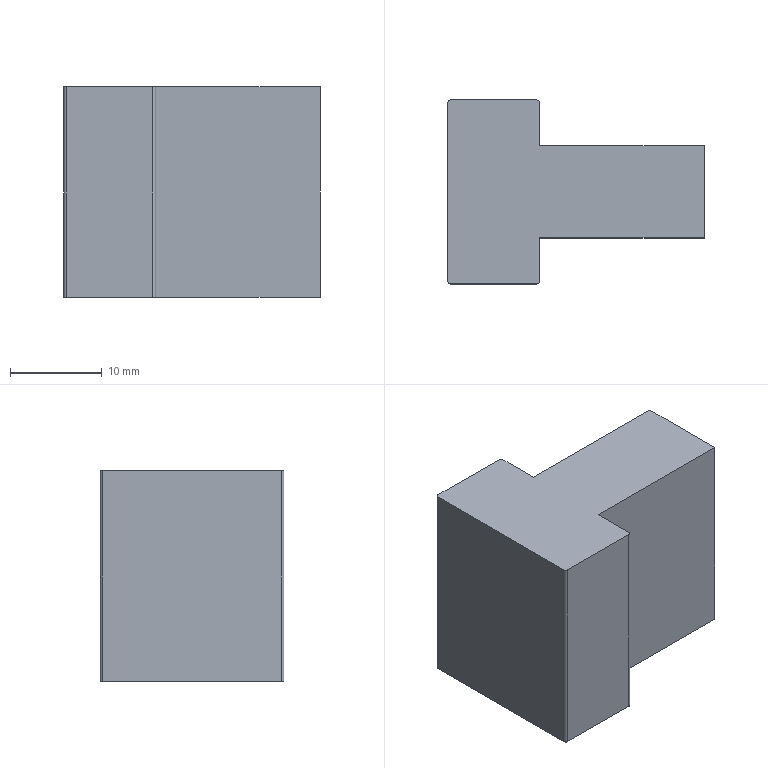Part | STEP file | 1 solid | 14 faces | box 27.92 x 20 x 22.9 mm | volume 8682 mm3 | plane 10 | cylinder 4 | commonest cylinder face diameters 0.6 x4
STEP:
#1=CARTESIAN_POINT('',(0.,0.,0.));
#2=DIRECTION('',(0.,0.,1.));
#3=DIRECTION('',(1.,0.,0.));
#4=AXIS2_PLACEMENT_3D('',#1,#2,#3);
#5=CARTESIAN_POINT('',(1582.157,369.98,23.619));
#6=VERTEX_POINT('',#5);
#7=CARTESIAN_POINT('',(1582.157,379.98,23.619));
#8=VERTEX_POINT('',#7);
#9=CARTESIAN_POINT('',(1582.157,384.68,23.619));
#10=DIRECTION('',(0.,1.,0.));
#11=VECTOR('',#10,1.);
#12=LINE('',#9,#11);
#13=CARTESIAN_POINT('',(1582.157,369.98,-0.381));
#14=DIRECTION('',(1.,0.,0.));
#15=DIRECTION('',(0.,-1.,0.));
#16=AXIS2_PLACEMENT_3D('',#13,#14,#15);
#17=PLANE('',#16);
#18=CARTESIAN_POINT('',(-14.7,-24.));
#19=DIRECTION('',(-1.,0.));
#20=VECTOR('',#19,1.);
#21=LINE('',#18,#20);
#22=(GEOMETRIC_REPRESENTATION_CONTEXT(2)PARAMETRIC_REPRESENTATION_CONTEXT()REPRESENTATION_CONTEXT('',''));
#23=DEFINITIONAL_REPRESENTATION('',(#21),#22);
#24=PCURVE('',#17,#23);
#25=CARTESIAN_POINT('',(1563.937,384.68,23.619));
#26=DIRECTION('',(0.,0.,1.));
#27=DIRECTION('',(-1.,0.,0.));
#28=AXIS2_PLACEMENT_3D('',#25,#26,#27);
#29=PLANE('',#28);
#30=CARTESIAN_POINT('',(-18.22,0.));
#31=DIRECTION('',(0.,-1.));
#32=VECTOR('',#31,1.);
#33=LINE('',#30,#32);
#34=(GEOMETRIC_REPRESENTATION_CONTEXT(2)PARAMETRIC_REPRESENTATION_CONTEXT()REPRESENTATION_CONTEXT('',''));
#35=DEFINITIONAL_REPRESENTATION('',(#33),#34);
#36=PCURVE('',#29,#35);
#37=SURFACE_CURVE('',#12,(#24,#36),.PCURVE_S1.);
#38=EDGE_CURVE('',#6,#8,#37,.T.);
#39=ORIENTED_EDGE('',*,*,#38,.F.);
#40=CARTESIAN_POINT('',(1582.157,369.98,0.719));
#41=VERTEX_POINT('',#40);
#42=CARTESIAN_POINT('',(1582.157,369.98,-0.381));
#43=DIRECTION('',(0.,0.,1.));
#44=VECTOR('',#43,1.);
#45=LINE('',#42,#44);
#46=CARTESIAN_POINT('',(0.,0.));
#47=DIRECTION('',(0.,-1.));
#48=VECTOR('',#47,1.);
#49=LINE('',#46,#48);
#50=(GEOMETRIC_REPRESENTATION_CONTEXT(2)PARAMETRIC_REPRESENTATION_CONTEXT()REPRESENTATION_CONTEXT('',''));
#51=DEFINITIONAL_REPRESENTATION('',(#49),#50);
#52=PCURVE('',#17,#51);
#53=CARTESIAN_POINT('',(1564.237,369.98,-0.381));
#54=DIRECTION('',(0.,-1.,0.));
#55=DIRECTION('',(0.,0.,-1.));
#56=AXIS2_PLACEMENT_3D('',#53,#54,#55);
#57=PLANE('',#56);
#58=CARTESIAN_POINT('',(0.,17.92));
#59=DIRECTION('',(-1.,0.));
#60=VECTOR('',#59,1.);
#61=LINE('',#58,#60);
#62=(GEOMETRIC_REPRESENTATION_CONTEXT(2)PARAMETRIC_REPRESENTATION_CONTEXT()REPRESENTATION_CONTEXT('',''));
#63=DEFINITIONAL_REPRESENTATION('',(#61),#62);
#64=PCURVE('',#57,#63);
#65=SURFACE_CURVE('',#45,(#52,#64),.PCURVE_S1.);
#66=EDGE_CURVE('',#41,#6,#65,.T.);
#67=ORIENTED_EDGE('',*,*,#66,.F.);
#68=CARTESIAN_POINT('',(1582.157,379.98,0.719));
#69=VERTEX_POINT('',#68);
#70=CARTESIAN_POINT('',(1582.157,369.98,0.719));
#71=DIRECTION('',(0.,1.,0.));
#72=VECTOR('',#71,1.);
#73=LINE('',#70,#72);
#74=CARTESIAN_POINT('',(0.,-1.1));
#75=DIRECTION('',(-1.,0.));
#76=VECTOR('',#75,1.);
#77=LINE('',#74,#76);
#78=(GEOMETRIC_REPRESENTATION_CONTEXT(2)PARAMETRIC_REPRESENTATION_CONTEXT()REPRESENTATION_CONTEXT('',''));
#79=DEFINITIONAL_REPRESENTATION('',(#77),#78);
#80=PCURVE('',#17,#79);
#81=CARTESIAN_POINT('',(1489.57,541.98,0.719));
#82=DIRECTION('',(0.,0.,-1.));
#83=DIRECTION('',(-1.,0.,0.));
#84=AXIS2_PLACEMENT_3D('',#81,#82,#83);
#85=PLANE('',#84);
#86=CARTESIAN_POINT('',(-92.587,-172.));
#87=DIRECTION('',(0.,1.));
#88=VECTOR('',#87,1.);
#89=LINE('',#86,#88);
#90=(GEOMETRIC_REPRESENTATION_CONTEXT(2)PARAMETRIC_REPRESENTATION_CONTEXT()REPRESENTATION_CONTEXT('',''));
#91=DEFINITIONAL_REPRESENTATION('',(#89),#90);
#92=PCURVE('',#85,#91);
#93=SURFACE_CURVE('',#73,(#80,#92),.PCURVE_S1.);
#94=EDGE_CURVE('',#41,#69,#93,.T.);
#95=ORIENTED_EDGE('',*,*,#94,.T.);
#96=CARTESIAN_POINT('',(1582.157,379.98,-0.381));
#97=DIRECTION('',(0.,0.,1.));
#98=VECTOR('',#97,1.);
#99=LINE('',#96,#98);
#100=CARTESIAN_POINT('',(-10.,0.));
#101=DIRECTION('',(0.,-1.));
#102=VECTOR('',#101,1.);
#103=LINE('',#100,#102);
#104=(GEOMETRIC_REPRESENTATION_CONTEXT(2)PARAMETRIC_REPRESENTATION_CONTEXT()REPRESENTATION_CONTEXT('',''));
#105=DEFINITIONAL_REPRESENTATION('',(#103),#104);
#106=PCURVE('',#17,#105);
#107=CARTESIAN_POINT('',(1577.237,379.98,-0.381));
#108=DIRECTION('',(0.,1.,0.));
#109=DIRECTION('',(0.,0.,1.));
#110=AXIS2_PLACEMENT_3D('',#107,#108,#109);
#111=PLANE('',#110);
#112=CARTESIAN_POINT('',(0.,4.92));
#113=DIRECTION('',(1.,0.));
#114=VECTOR('',#113,1.);
#115=LINE('',#112,#114);
#116=(GEOMETRIC_REPRESENTATION_CONTEXT(2)PARAMETRIC_REPRESENTATION_CONTEXT()REPRESENTATION_CONTEXT('',''));
#117=DEFINITIONAL_REPRESENTATION('',(#115),#116);
#118=PCURVE('',#111,#117);
#119=SURFACE_CURVE('',#99,(#106,#118),.PCURVE_S1.);
#120=EDGE_CURVE('',#69,#8,#119,.T.);
#121=ORIENTED_EDGE('',*,*,#120,.T.);
#122=EDGE_LOOP('',(#39,#67,#95,#121));
#123=FACE_BOUND('',#122,.T.);
#124=ADVANCED_FACE('',(#123),#17,.T.);
#125=CARTESIAN_POINT('',(1564.237,379.98,23.619));
#126=VERTEX_POINT('',#125);
#127=CARTESIAN_POINT('',(1577.237,379.98,23.619));
#128=DIRECTION('',(-1.,0.,0.));
#129=VECTOR('',#128,1.);
#130=LINE('',#127,#129);
#131=CARTESIAN_POINT('',(24.,0.));
#132=DIRECTION('',(0.,-1.));
#133=VECTOR('',#132,1.);
#134=LINE('',#131,#133);
#135=(GEOMETRIC_REPRESENTATION_CONTEXT(2)PARAMETRIC_REPRESENTATION_CONTEXT()REPRESENTATION_CONTEXT('',''));
#136=DEFINITIONAL_REPRESENTATION('',(#134),#135);
#137=PCURVE('',#111,#136);
#138=CARTESIAN_POINT('',(-13.3,4.7));
#139=DIRECTION('',(1.,0.));
#140=VECTOR('',#139,1.);
#141=LINE('',#138,#140);
#142=(GEOMETRIC_REPRESENTATION_CONTEXT(2)PARAMETRIC_REPRESENTATION_CONTEXT()REPRESENTATION_CONTEXT('',''));
#143=DEFINITIONAL_REPRESENTATION('',(#141),#142);
#144=PCURVE('',#29,#143);
#145=SURFACE_CURVE('',#130,(#137,#144),.PCURVE_S1.);
#146=EDGE_CURVE('',#8,#126,#145,.T.);
#147=ORIENTED_EDGE('',*,*,#146,.F.);
#148=ORIENTED_EDGE('',*,*,#120,.F.);
#149=CARTESIAN_POINT('',(1564.237,379.98,0.719));
#150=VERTEX_POINT('',#149);
#151=CARTESIAN_POINT('',(1489.57,379.98,0.719));
#152=DIRECTION('',(-1.,0.,0.));
#153=VECTOR('',#152,1.);
#154=LINE('',#151,#153);
#155=CARTESIAN_POINT('',(1.1,-87.667));
#156=DIRECTION('',(0.,-1.));
#157=VECTOR('',#156,1.);
#158=LINE('',#155,#157);
#159=(GEOMETRIC_REPRESENTATION_CONTEXT(2)PARAMETRIC_REPRESENTATION_CONTEXT()REPRESENTATION_CONTEXT('',''));
#160=DEFINITIONAL_REPRESENTATION('',(#158),#159);
#161=PCURVE('',#111,#160);
#162=CARTESIAN_POINT('',(0.,-162.));
#163=DIRECTION('',(1.,0.));
#164=VECTOR('',#163,1.);
#165=LINE('',#162,#164);
#166=(GEOMETRIC_REPRESENTATION_CONTEXT(2)PARAMETRIC_REPRESENTATION_CONTEXT()REPRESENTATION_CONTEXT('',''));
#167=DEFINITIONAL_REPRESENTATION('',(#165),#166);
#168=PCURVE('',#85,#167);
#169=SURFACE_CURVE('',#154,(#161,#168),.PCURVE_S1.);
#170=EDGE_CURVE('',#69,#150,#169,.T.);
#171=ORIENTED_EDGE('',*,*,#170,.T.);
#172=CARTESIAN_POINT('',(1564.237,379.98,-0.381));
#173=DIRECTION('',(0.,0.,1.));
#174=VECTOR('',#173,1.);
#175=LINE('',#172,#174);
#176=CARTESIAN_POINT('',(0.,-13.));
#177=DIRECTION('',(1.,0.));
#178=VECTOR('',#177,1.);
#179=LINE('',#176,#178);
#180=(GEOMETRIC_REPRESENTATION_CONTEXT(2)PARAMETRIC_REPRESENTATION_CONTEXT()REPRESENTATION_CONTEXT('',''));
#181=DEFINITIONAL_REPRESENTATION('',(#179),#180);
#182=PCURVE('',#111,#181);
#183=CARTESIAN_POINT('',(1564.237,379.98,-0.381));
#184=DIRECTION('',(1.,0.,0.));
#185=DIRECTION('',(0.,0.,1.));
#186=AXIS2_PLACEMENT_3D('',#183,#184,#185);
#187=PLANE('',#186);
#188=CARTESIAN_POINT('',(0.,0.));
#189=DIRECTION('',(1.,0.));
#190=VECTOR('',#189,1.);
#191=LINE('',#188,#190);
#192=(GEOMETRIC_REPRESENTATION_CONTEXT(2)PARAMETRIC_REPRESENTATION_CONTEXT()REPRESENTATION_CONTEXT('',''));
#193=DEFINITIONAL_REPRESENTATION('',(#191),#192);
#194=PCURVE('',#187,#193);
#195=SURFACE_CURVE('',#175,(#182,#194),.PCURVE_S1.);
#196=EDGE_CURVE('',#150,#126,#195,.T.);
#197=ORIENTED_EDGE('',*,*,#196,.T.);
#198=EDGE_LOOP('',(#147,#148,#171,#197));
#199=FACE_BOUND('',#198,.T.);
#200=ADVANCED_FACE('',(#199),#111,.T.);
#201=CARTESIAN_POINT('',(1564.237,384.68,23.619));
#202=VERTEX_POINT('',#201);
#203=CARTESIAN_POINT('',(1564.237,379.98,23.619));
#204=DIRECTION('',(0.,1.,0.));
#205=VECTOR('',#204,1.);
#206=LINE('',#203,#205);
#207=CARTESIAN_POINT('',(24.,0.));
#208=DIRECTION('',(0.,-1.));
#209=VECTOR('',#208,1.);
#210=LINE('',#207,#209);
#211=(GEOMETRIC_REPRESENTATION_CONTEXT(2)PARAMETRIC_REPRESENTATION_CONTEXT()REPRESENTATION_CONTEXT('',''));
#212=DEFINITIONAL_REPRESENTATION('',(#210),#211);
#213=PCURVE('',#187,#212);
#214=CARTESIAN_POINT('',(-0.3,4.7));
#215=DIRECTION('',(0.,-1.));
#216=VECTOR('',#215,1.);
#217=LINE('',#214,#216);
#218=(GEOMETRIC_REPRESENTATION_CONTEXT(2)PARAMETRIC_REPRESENTATION_CONTEXT()REPRESENTATION_CONTEXT('',''));
#219=DEFINITIONAL_REPRESENTATION('',(#217),#218);
#220=PCURVE('',#29,#219);
#221=SURFACE_CURVE('',#206,(#213,#220),.PCURVE_S1.);
#222=EDGE_CURVE('',#126,#202,#221,.T.);
#223=ORIENTED_EDGE('',*,*,#222,.F.);
#224=ORIENTED_EDGE('',*,*,#196,.F.);
#225=CARTESIAN_POINT('',(1564.237,384.68,0.719));
#226=VERTEX_POINT('',#225);
#227=CARTESIAN_POINT('',(1564.237,541.98,0.719));
#228=DIRECTION('',(0.,1.,0.));
#229=VECTOR('',#228,1.);
#230=LINE('',#227,#229);
#231=CARTESIAN_POINT('',(1.1,-162.));
#232=DIRECTION('',(0.,-1.));
#233=VECTOR('',#232,1.);
#234=LINE('',#231,#233);
#235=(GEOMETRIC_REPRESENTATION_CONTEXT(2)PARAMETRIC_REPRESENTATION_CONTEXT()REPRESENTATION_CONTEXT('',''));
#236=DEFINITIONAL_REPRESENTATION('',(#234),#235);
#237=PCURVE('',#187,#236);
#238=CARTESIAN_POINT('',(-74.667,0.));
#239=DIRECTION('',(0.,1.));
#240=VECTOR('',#239,1.);
#241=LINE('',#238,#240);
#242=(GEOMETRIC_REPRESENTATION_CONTEXT(2)PARAMETRIC_REPRESENTATION_CONTEXT()REPRESENTATION_CONTEXT('',''));
#243=DEFINITIONAL_REPRESENTATION('',(#241),#242);
#244=PCURVE('',#85,#243);
#245=SURFACE_CURVE('',#230,(#237,#244),.PCURVE_S1.);
#246=EDGE_CURVE('',#150,#226,#245,.T.);
#247=ORIENTED_EDGE('',*,*,#246,.T.);
#248=CARTESIAN_POINT('',(1564.237,384.68,-0.381));
#249=DIRECTION('',(0.,0.,1.));
#250=VECTOR('',#249,1.);
#251=LINE('',#248,#250);
#252=CARTESIAN_POINT('',(0.,-4.7));
#253=DIRECTION('',(1.,0.));
#254=VECTOR('',#253,1.);
#255=LINE('',#252,#254);
#256=(GEOMETRIC_REPRESENTATION_CONTEXT(2)PARAMETRIC_REPRESENTATION_CONTEXT()REPRESENTATION_CONTEXT('',''));
#257=DEFINITIONAL_REPRESENTATION('',(#255),#256);
#258=PCURVE('',#187,#257);
#259=CARTESIAN_POINT('',(1563.937,384.68,-0.381));
#260=DIRECTION('',(0.,0.,1.));
#261=DIRECTION('',(-1.,0.,0.));
#262=AXIS2_PLACEMENT_3D('',#259,#260,#261);
#263=CYLINDRICAL_SURFACE('',#262,0.3);
#264=CARTESIAN_POINT('',(3.142,0.));
#265=DIRECTION('',(0.,1.));
#266=VECTOR('',#265,1.);
#267=LINE('',#264,#266);
#268=(GEOMETRIC_REPRESENTATION_CONTEXT(2)PARAMETRIC_REPRESENTATION_CONTEXT()REPRESENTATION_CONTEXT('',''));
#269=DEFINITIONAL_REPRESENTATION('',(#267),#268);
#270=PCURVE('',#263,#269);
#271=SURFACE_CURVE('',#251,(#258,#270),.PCURVE_S1.);
#272=EDGE_CURVE('',#226,#202,#271,.T.);
#273=ORIENTED_EDGE('',*,*,#272,.T.);
#274=EDGE_LOOP('',(#223,#224,#247,#273));
#275=FACE_BOUND('',#274,.T.);
#276=ADVANCED_FACE('',(#275),#187,.T.);
#277=CARTESIAN_POINT('',(1563.937,384.98,23.619));
#278=VERTEX_POINT('',#277);
#279=CARTESIAN_POINT('',(1563.937,384.68,23.619));
#280=DIRECTION('',(0.,0.,1.));
#281=DIRECTION('',(1.,0.,0.));
#282=AXIS2_PLACEMENT_3D('',#279,#280,#281);
#283=CIRCLE('',#282,0.3);
#284=CARTESIAN_POINT('',(3.142,24.));
#285=DIRECTION('',(1.,0.));
#286=VECTOR('',#285,1.);
#287=LINE('',#284,#286);
#288=(GEOMETRIC_REPRESENTATION_CONTEXT(2)PARAMETRIC_REPRESENTATION_CONTEXT()REPRESENTATION_CONTEXT('',''));
#289=DEFINITIONAL_REPRESENTATION('',(#287),#288);
#290=PCURVE('',#263,#289);
#291=CARTESIAN_POINT('',(0.,0.));
#292=DIRECTION('',(-1.,0.));
#293=AXIS2_PLACEMENT_2D('',#291,#292);
#294=CIRCLE('',#293,0.3);
#295=(GEOMETRIC_REPRESENTATION_CONTEXT(2)PARAMETRIC_REPRESENTATION_CONTEXT()REPRESENTATION_CONTEXT('',''));
#296=DEFINITIONAL_REPRESENTATION('',(#294),#295);
#297=PCURVE('',#29,#296);
#298=SURFACE_CURVE('',#283,(#290,#297),.PCURVE_S1.);
#299=EDGE_CURVE('',#202,#278,#298,.T.);
#300=ORIENTED_EDGE('',*,*,#299,.F.);
#301=ORIENTED_EDGE('',*,*,#272,.F.);
#302=CARTESIAN_POINT('',(1563.937,384.98,0.719));
#303=VERTEX_POINT('',#302);
#304=CARTESIAN_POINT('',(1563.937,384.68,0.719));
#305=DIRECTION('',(0.,0.,1.));
#306=DIRECTION('',(1.,0.,0.));
#307=AXIS2_PLACEMENT_3D('',#304,#305,#306);
#308=CIRCLE('',#307,0.3);
#309=CARTESIAN_POINT('',(3.142,1.1));
#310=DIRECTION('',(1.,0.));
#311=VECTOR('',#310,1.);
#312=LINE('',#309,#311);
#313=(GEOMETRIC_REPRESENTATION_CONTEXT(2)PARAMETRIC_REPRESENTATION_CONTEXT()REPRESENTATION_CONTEXT('',''));
#314=DEFINITIONAL_REPRESENTATION('',(#312),#313);
#315=PCURVE('',#263,#314);
#316=CARTESIAN_POINT('',(-74.667,-157.3));
#317=CARTESIAN_POINT('',(-74.667,-156.78));
#318=CARTESIAN_POINT('',(-74.217,-157.04));
#319=CARTESIAN_POINT('',(-73.767,-157.3));
#320=CARTESIAN_POINT('',(-74.217,-157.56));
#321=CARTESIAN_POINT('',(-74.667,-157.82));
#322=CARTESIAN_POINT('',(-74.667,-157.3));
#323=(BOUNDED_CURVE()B_SPLINE_CURVE(2,(#316,#317,#318,#319,#320,#321,#322),.UNSPECIFIED.,.T.,.F.)B_SPLINE_CURVE_WITH_KNOTS((1,2,2,2,2,1),(-2.094,0.,2.094,4.189,6.283,8.378),.UNSPECIFIED.)CURVE()GEOMETRIC_REPRESENTATION_ITEM()RATIONAL_B_SPLINE_CURVE((1.,0.5,1.,0.5,1.,0.5,1.))REPRESENTATION_ITEM(''));
#324=(GEOMETRIC_REPRESENTATION_CONTEXT(2)PARAMETRIC_REPRESENTATION_CONTEXT()REPRESENTATION_CONTEXT('',''));
#325=DEFINITIONAL_REPRESENTATION('',(#323),#324);
#326=PCURVE('',#85,#325);
#327=SURFACE_CURVE('',#308,(#315,#326),.PCURVE_S1.);
#328=EDGE_CURVE('',#226,#303,#327,.T.);
#329=ORIENTED_EDGE('',*,*,#328,.T.);
#330=CARTESIAN_POINT('',(1563.937,384.98,-0.381));
#331=DIRECTION('',(0.,0.,1.));
#332=VECTOR('',#331,1.);
#333=LINE('',#330,#332);
#334=CARTESIAN_POINT('',(4.712,0.));
#335=DIRECTION('',(0.,1.));
#336=VECTOR('',#335,1.);
#337=LINE('',#334,#336);
#338=(GEOMETRIC_REPRESENTATION_CONTEXT(2)PARAMETRIC_REPRESENTATION_CONTEXT()REPRESENTATION_CONTEXT('',''));
#339=DEFINITIONAL_REPRESENTATION('',(#337),#338);
#340=PCURVE('',#263,#339);
#341=CARTESIAN_POINT('',(1563.937,384.98,-0.381));
#342=DIRECTION('',(0.,1.,0.));
#343=DIRECTION('',(0.,0.,1.));
#344=AXIS2_PLACEMENT_3D('',#341,#342,#343);
#345=PLANE('',#344);
#346=CARTESIAN_POINT('',(0.,0.));
#347=DIRECTION('',(1.,0.));
#348=VECTOR('',#347,1.);
#349=LINE('',#346,#348);
#350=(GEOMETRIC_REPRESENTATION_CONTEXT(2)PARAMETRIC_REPRESENTATION_CONTEXT()REPRESENTATION_CONTEXT('',''));
#351=DEFINITIONAL_REPRESENTATION('',(#349),#350);
#352=PCURVE('',#345,#351);
#353=SURFACE_CURVE('',#333,(#340,#352),.PCURVE_S1.);
#354=EDGE_CURVE('',#303,#278,#353,.T.);
#355=ORIENTED_EDGE('',*,*,#354,.T.);
#356=EDGE_LOOP('',(#300,#301,#329,#355));
#357=FACE_BOUND('',#356,.T.);
#358=ADVANCED_FACE('',(#357),#263,.T.);
#359=CARTESIAN_POINT('',(1554.537,384.98,23.619));
#360=VERTEX_POINT('',#359);
#361=CARTESIAN_POINT('',(1563.937,384.98,23.619));
#362=DIRECTION('',(-1.,0.,0.));
#363=VECTOR('',#362,1.);
#364=LINE('',#361,#363);
#365=CARTESIAN_POINT('',(24.,0.));
#366=DIRECTION('',(0.,-1.));
#367=VECTOR('',#366,1.);
#368=LINE('',#365,#367);
#369=(GEOMETRIC_REPRESENTATION_CONTEXT(2)PARAMETRIC_REPRESENTATION_CONTEXT()REPRESENTATION_CONTEXT('',''));
#370=DEFINITIONAL_REPRESENTATION('',(#368),#369);
#371=PCURVE('',#345,#370);
#372=CARTESIAN_POINT('',(0.,-0.3));
#373=DIRECTION('',(1.,0.));
#374=VECTOR('',#373,1.);
#375=LINE('',#372,#374);
#376=(GEOMETRIC_REPRESENTATION_CONTEXT(2)PARAMETRIC_REPRESENTATION_CONTEXT()REPRESENTATION_CONTEXT('',''));
#377=DEFINITIONAL_REPRESENTATION('',(#375),#376);
#378=PCURVE('',#29,#377);
#379=SURFACE_CURVE('',#364,(#371,#378),.PCURVE_S1.);
#380=EDGE_CURVE('',#278,#360,#379,.T.);
#381=ORIENTED_EDGE('',*,*,#380,.F.);
#382=ORIENTED_EDGE('',*,*,#354,.F.);
#383=CARTESIAN_POINT('',(1554.537,384.98,0.719));
#384=VERTEX_POINT('',#383);
#385=CARTESIAN_POINT('',(1489.57,384.98,0.719));
#386=DIRECTION('',(-1.,0.,0.));
#387=VECTOR('',#386,1.);
#388=LINE('',#385,#387);
#389=CARTESIAN_POINT('',(1.1,-74.367));
#390=DIRECTION('',(0.,-1.));
#391=VECTOR('',#390,1.);
#392=LINE('',#389,#391);
#393=(GEOMETRIC_REPRESENTATION_CONTEXT(2)PARAMETRIC_REPRESENTATION_CONTEXT()REPRESENTATION_CONTEXT('',''));
#394=DEFINITIONAL_REPRESENTATION('',(#392),#393);
#395=PCURVE('',#345,#394);
#396=CARTESIAN_POINT('',(0.,-157.));
#397=DIRECTION('',(1.,0.));
#398=VECTOR('',#397,1.);
#399=LINE('',#396,#398);
#400=(GEOMETRIC_REPRESENTATION_CONTEXT(2)PARAMETRIC_REPRESENTATION_CONTEXT()REPRESENTATION_CONTEXT('',''));
#401=DEFINITIONAL_REPRESENTATION('',(#399),#400);
#402=PCURVE('',#85,#401);
#403=SURFACE_CURVE('',#388,(#395,#402),.PCURVE_S1.);
#404=EDGE_CURVE('',#303,#384,#403,.T.);
#405=ORIENTED_EDGE('',*,*,#404,.T.);
#406=CARTESIAN_POINT('',(1554.537,384.98,-0.381));
#407=DIRECTION('',(0.,0.,1.));
#408=VECTOR('',#407,1.);
#409=LINE('',#406,#408);
#410=CARTESIAN_POINT('',(0.,-9.4));
#411=DIRECTION('',(1.,0.));
#412=VECTOR('',#411,1.);
#413=LINE('',#410,#412);
#414=(GEOMETRIC_REPRESENTATION_CONTEXT(2)PARAMETRIC_REPRESENTATION_CONTEXT()REPRESENTATION_CONTEXT('',''));
#415=DEFINITIONAL_REPRESENTATION('',(#413),#414);
#416=PCURVE('',#345,#415);
#417=CARTESIAN_POINT('',(1554.537,384.68,-0.381));
#418=DIRECTION('',(0.,0.,1.));
#419=DIRECTION('',(-1.,0.,0.));
#420=AXIS2_PLACEMENT_3D('',#417,#418,#419);
#421=CYLINDRICAL_SURFACE('',#420,0.3);
#422=CARTESIAN_POINT('',(4.712,0.));
#423=DIRECTION('',(0.,1.));
#424=VECTOR('',#423,1.);
#425=LINE('',#422,#424);
#426=(GEOMETRIC_REPRESENTATION_CONTEXT(2)PARAMETRIC_REPRESENTATION_CONTEXT()REPRESENTATION_CONTEXT('',''));
#427=DEFINITIONAL_REPRESENTATION('',(#425),#426);
#428=PCURVE('',#421,#427);
#429=SURFACE_CURVE('',#409,(#416,#428),.PCURVE_S1.);
#430=EDGE_CURVE('',#384,#360,#429,.T.);
#431=ORIENTED_EDGE('',*,*,#430,.T.);
#432=EDGE_LOOP('',(#381,#382,#405,#431));
#433=FACE_BOUND('',#432,.T.);
#434=ADVANCED_FACE('',(#433),#345,.T.);
#435=CARTESIAN_POINT('',(1554.237,384.68,23.619));
#436=VERTEX_POINT('',#435);
#437=CARTESIAN_POINT('',(1554.537,384.68,23.619));
#438=DIRECTION('',(0.,0.,1.));
#439=DIRECTION('',(1.,0.,0.));
#440=AXIS2_PLACEMENT_3D('',#437,#438,#439);
#441=CIRCLE('',#440,0.3);
#442=CARTESIAN_POINT('',(3.142,24.));
#443=DIRECTION('',(1.,0.));
#444=VECTOR('',#443,1.);
#445=LINE('',#442,#444);
#446=(GEOMETRIC_REPRESENTATION_CONTEXT(2)PARAMETRIC_REPRESENTATION_CONTEXT()REPRESENTATION_CONTEXT('',''));
#447=DEFINITIONAL_REPRESENTATION('',(#445),#446);
#448=PCURVE('',#421,#447);
#449=CARTESIAN_POINT('',(9.4,0.));
#450=DIRECTION('',(-1.,0.));
#451=AXIS2_PLACEMENT_2D('',#449,#450);
#452=CIRCLE('',#451,0.3);
#453=(GEOMETRIC_REPRESENTATION_CONTEXT(2)PARAMETRIC_REPRESENTATION_CONTEXT()REPRESENTATION_CONTEXT('',''));
#454=DEFINITIONAL_REPRESENTATION('',(#452),#453);
#455=PCURVE('',#29,#454);
#456=SURFACE_CURVE('',#441,(#448,#455),.PCURVE_S1.);
#457=EDGE_CURVE('',#360,#436,#456,.T.);
#458=ORIENTED_EDGE('',*,*,#457,.F.);
#459=ORIENTED_EDGE('',*,*,#430,.F.);
#460=CARTESIAN_POINT('',(1554.237,384.68,0.719));
#461=VERTEX_POINT('',#460);
#462=CARTESIAN_POINT('',(1554.537,384.68,0.719));
#463=DIRECTION('',(0.,0.,1.));
#464=DIRECTION('',(1.,0.,0.));
#465=AXIS2_PLACEMENT_3D('',#462,#463,#464);
#466=CIRCLE('',#465,0.3);
#467=CARTESIAN_POINT('',(3.142,1.1));
#468=DIRECTION('',(1.,0.));
#469=VECTOR('',#468,1.);
#470=LINE('',#467,#469);
#471=(GEOMETRIC_REPRESENTATION_CONTEXT(2)PARAMETRIC_REPRESENTATION_CONTEXT()REPRESENTATION_CONTEXT('',''));
#472=DEFINITIONAL_REPRESENTATION('',(#470),#471);
#473=PCURVE('',#421,#472);
#474=CARTESIAN_POINT('',(-65.267,-157.3));
#475=CARTESIAN_POINT('',(-65.267,-156.78));
#476=CARTESIAN_POINT('',(-64.817,-157.04));
#477=CARTESIAN_POINT('',(-64.367,-157.3));
#478=CARTESIAN_POINT('',(-64.817,-157.56));
#479=CARTESIAN_POINT('',(-65.267,-157.82));
#480=CARTESIAN_POINT('',(-65.267,-157.3));
#481=(BOUNDED_CURVE()B_SPLINE_CURVE(2,(#474,#475,#476,#477,#478,#479,#480),.UNSPECIFIED.,.T.,.F.)B_SPLINE_CURVE_WITH_KNOTS((1,2,2,2,2,1),(-2.094,0.,2.094,4.189,6.283,8.378),.UNSPECIFIED.)CURVE()GEOMETRIC_REPRESENTATION_ITEM()RATIONAL_B_SPLINE_CURVE((1.,0.5,1.,0.5,1.,0.5,1.))REPRESENTATION_ITEM(''));
#482=(GEOMETRIC_REPRESENTATION_CONTEXT(2)PARAMETRIC_REPRESENTATION_CONTEXT()REPRESENTATION_CONTEXT('',''));
#483=DEFINITIONAL_REPRESENTATION('',(#481),#482);
#484=PCURVE('',#85,#483);
#485=SURFACE_CURVE('',#466,(#473,#484),.PCURVE_S1.);
#486=EDGE_CURVE('',#384,#461,#485,.T.);
#487=ORIENTED_EDGE('',*,*,#486,.T.);
#488=CARTESIAN_POINT('',(1554.237,384.68,-0.381));
#489=DIRECTION('',(0.,0.,1.));
#490=VECTOR('',#489,1.);
#491=LINE('',#488,#490);
#492=CARTESIAN_POINT('',(6.283,0.));
#493=DIRECTION('',(0.,1.));
#494=VECTOR('',#493,1.);
#495=LINE('',#492,#494);
#496=(GEOMETRIC_REPRESENTATION_CONTEXT(2)PARAMETRIC_REPRESENTATION_CONTEXT()REPRESENTATION_CONTEXT('',''));
#497=DEFINITIONAL_REPRESENTATION('',(#495),#496);
#498=PCURVE('',#421,#497);
#499=CARTESIAN_POINT('',(1554.237,384.68,-0.381));
#500=DIRECTION('',(-1.,0.,0.));
#501=DIRECTION('',(0.,0.,-1.));
#502=AXIS2_PLACEMENT_3D('',#499,#500,#501);
#503=PLANE('',#502);
#504=CARTESIAN_POINT('',(0.,0.));
#505=DIRECTION('',(-1.,0.));
#506=VECTOR('',#505,1.);
#507=LINE('',#504,#506);
#508=(GEOMETRIC_REPRESENTATION_CONTEXT(2)PARAMETRIC_REPRESENTATION_CONTEXT()REPRESENTATION_CONTEXT('',''));
#509=DEFINITIONAL_REPRESENTATION('',(#507),#508);
#510=PCURVE('',#503,#509);
#511=SURFACE_CURVE('',#491,(#498,#510),.PCURVE_S1.);
#512=EDGE_CURVE('',#461,#436,#511,.T.);
#513=ORIENTED_EDGE('',*,*,#512,.T.);
#514=EDGE_LOOP('',(#458,#459,#487,#513));
#515=FACE_BOUND('',#514,.T.);
#516=ADVANCED_FACE('',(#515),#421,.T.);
#517=CARTESIAN_POINT('',(1554.237,365.28,23.619));
#518=VERTEX_POINT('',#517);
#519=CARTESIAN_POINT('',(1554.237,384.68,23.619));
#520=DIRECTION('',(0.,-1.,0.));
#521=VECTOR('',#520,1.);
#522=LINE('',#519,#521);
#523=CARTESIAN_POINT('',(-24.,0.));
#524=DIRECTION('',(0.,1.));
#525=VECTOR('',#524,1.);
#526=LINE('',#523,#525);
#527=(GEOMETRIC_REPRESENTATION_CONTEXT(2)PARAMETRIC_REPRESENTATION_CONTEXT()REPRESENTATION_CONTEXT('',''));
#528=DEFINITIONAL_REPRESENTATION('',(#526),#527);
#529=PCURVE('',#503,#528);
#530=CARTESIAN_POINT('',(9.7,0.));
#531=DIRECTION('',(0.,1.));
#532=VECTOR('',#531,1.);
#533=LINE('',#530,#532);
#534=(GEOMETRIC_REPRESENTATION_CONTEXT(2)PARAMETRIC_REPRESENTATION_CONTEXT()REPRESENTATION_CONTEXT('',''));
#535=DEFINITIONAL_REPRESENTATION('',(#533),#534);
#536=PCURVE('',#29,#535);
#537=SURFACE_CURVE('',#522,(#529,#536),.PCURVE_S1.);
#538=EDGE_CURVE('',#436,#518,#537,.T.);
#539=ORIENTED_EDGE('',*,*,#538,.F.);
#540=ORIENTED_EDGE('',*,*,#512,.F.);
#541=CARTESIAN_POINT('',(1554.237,365.28,0.719));
#542=VERTEX_POINT('',#541);
#543=CARTESIAN_POINT('',(1554.237,541.98,0.719));
#544=DIRECTION('',(0.,-1.,0.));
#545=VECTOR('',#544,1.);
#546=LINE('',#543,#545);
#547=CARTESIAN_POINT('',(-1.1,-157.3));
#548=DIRECTION('',(0.,1.));
#549=VECTOR('',#548,1.);
#550=LINE('',#547,#549);
#551=(GEOMETRIC_REPRESENTATION_CONTEXT(2)PARAMETRIC_REPRESENTATION_CONTEXT()REPRESENTATION_CONTEXT('',''));
#552=DEFINITIONAL_REPRESENTATION('',(#550),#551);
#553=PCURVE('',#503,#552);
#554=CARTESIAN_POINT('',(-64.667,0.));
#555=DIRECTION('',(0.,-1.));
#556=VECTOR('',#555,1.);
#557=LINE('',#554,#556);
#558=(GEOMETRIC_REPRESENTATION_CONTEXT(2)PARAMETRIC_REPRESENTATION_CONTEXT()REPRESENTATION_CONTEXT('',''));
#559=DEFINITIONAL_REPRESENTATION('',(#557),#558);
#560=PCURVE('',#85,#559);
#561=SURFACE_CURVE('',#546,(#553,#560),.PCURVE_S1.);
#562=EDGE_CURVE('',#461,#542,#561,.T.);
#563=ORIENTED_EDGE('',*,*,#562,.T.);
#564=CARTESIAN_POINT('',(1554.237,365.28,-0.381));
#565=DIRECTION('',(0.,0.,1.));
#566=VECTOR('',#565,1.);
#567=LINE('',#564,#566);
#568=CARTESIAN_POINT('',(0.,19.4));
#569=DIRECTION('',(-1.,0.));
#570=VECTOR('',#569,1.);
#571=LINE('',#568,#570);
#572=(GEOMETRIC_REPRESENTATION_CONTEXT(2)PARAMETRIC_REPRESENTATION_CONTEXT()REPRESENTATION_CONTEXT('',''));
#573=DEFINITIONAL_REPRESENTATION('',(#571),#572);
#574=PCURVE('',#503,#573);
#575=CARTESIAN_POINT('',(1554.537,365.28,-0.381));
#576=DIRECTION('',(0.,0.,1.));
#577=DIRECTION('',(-1.,0.,0.));
#578=AXIS2_PLACEMENT_3D('',#575,#576,#577);
#579=CYLINDRICAL_SURFACE('',#578,0.3);
#580=CARTESIAN_POINT('',(0.,0.));
#581=DIRECTION('',(0.,1.));
#582=VECTOR('',#581,1.);
#583=LINE('',#580,#582);
#584=(GEOMETRIC_REPRESENTATION_CONTEXT(2)PARAMETRIC_REPRESENTATION_CONTEXT()REPRESENTATION_CONTEXT('',''));
#585=DEFINITIONAL_REPRESENTATION('',(#583),#584);
#586=PCURVE('',#579,#585);
#587=SURFACE_CURVE('',#567,(#574,#586),.PCURVE_S1.);
#588=EDGE_CURVE('',#542,#518,#587,.T.);
#589=ORIENTED_EDGE('',*,*,#588,.T.);
#590=EDGE_LOOP('',(#539,#540,#563,#589));
#591=FACE_BOUND('',#590,.T.);
#592=ADVANCED_FACE('',(#591),#503,.T.);
#593=CARTESIAN_POINT('',(1554.537,364.98,23.619));
#594=VERTEX_POINT('',#593);
#595=CARTESIAN_POINT('',(1554.537,365.28,23.619));
#596=DIRECTION('',(0.,0.,1.));
#597=DIRECTION('',(1.,0.,0.));
#598=AXIS2_PLACEMENT_3D('',#595,#596,#597);
#599=CIRCLE('',#598,0.3);
#600=CARTESIAN_POINT('',(-3.142,24.));
#601=DIRECTION('',(1.,0.));
#602=VECTOR('',#601,1.);
#603=LINE('',#600,#602);
#604=(GEOMETRIC_REPRESENTATION_CONTEXT(2)PARAMETRIC_REPRESENTATION_CONTEXT()REPRESENTATION_CONTEXT('',''));
#605=DEFINITIONAL_REPRESENTATION('',(#603),#604);
#606=PCURVE('',#579,#605);
#607=CARTESIAN_POINT('',(9.4,19.4));
#608=DIRECTION('',(-1.,0.));
#609=AXIS2_PLACEMENT_2D('',#607,#608);
#610=CIRCLE('',#609,0.3);
#611=(GEOMETRIC_REPRESENTATION_CONTEXT(2)PARAMETRIC_REPRESENTATION_CONTEXT()REPRESENTATION_CONTEXT('',''));
#612=DEFINITIONAL_REPRESENTATION('',(#610),#611);
#613=PCURVE('',#29,#612);
#614=SURFACE_CURVE('',#599,(#606,#613),.PCURVE_S1.);
#615=EDGE_CURVE('',#518,#594,#614,.T.);
#616=ORIENTED_EDGE('',*,*,#615,.F.);
#617=ORIENTED_EDGE('',*,*,#588,.F.);
#618=CARTESIAN_POINT('',(1554.537,364.98,0.719));
#619=VERTEX_POINT('',#618);
#620=CARTESIAN_POINT('',(1554.537,365.28,0.719));
#621=DIRECTION('',(0.,0.,1.));
#622=DIRECTION('',(1.,0.,0.));
#623=AXIS2_PLACEMENT_3D('',#620,#621,#622);
#624=CIRCLE('',#623,0.3);
#625=CARTESIAN_POINT('',(-3.142,1.1));
#626=DIRECTION('',(1.,0.));
#627=VECTOR('',#626,1.);
#628=LINE('',#625,#627);
#629=(GEOMETRIC_REPRESENTATION_CONTEXT(2)PARAMETRIC_REPRESENTATION_CONTEXT()REPRESENTATION_CONTEXT('',''));
#630=DEFINITIONAL_REPRESENTATION('',(#628),#629);
#631=PCURVE('',#579,#630);
#632=CARTESIAN_POINT('',(-65.267,-176.7));
#633=CARTESIAN_POINT('',(-65.267,-176.18));
#634=CARTESIAN_POINT('',(-64.817,-176.44));
#635=CARTESIAN_POINT('',(-64.367,-176.7));
#636=CARTESIAN_POINT('',(-64.817,-176.96));
#637=CARTESIAN_POINT('',(-65.267,-177.22));
#638=CARTESIAN_POINT('',(-65.267,-176.7));
#639=(BOUNDED_CURVE()B_SPLINE_CURVE(2,(#632,#633,#634,#635,#636,#637,#638),.UNSPECIFIED.,.T.,.F.)B_SPLINE_CURVE_WITH_KNOTS((1,2,2,2,2,1),(-2.094,0.,2.094,4.189,6.283,8.378),.UNSPECIFIED.)CURVE()GEOMETRIC_REPRESENTATION_ITEM()RATIONAL_B_SPLINE_CURVE((1.,0.5,1.,0.5,1.,0.5,1.))REPRESENTATION_ITEM(''));
#640=(GEOMETRIC_REPRESENTATION_CONTEXT(2)PARAMETRIC_REPRESENTATION_CONTEXT()REPRESENTATION_CONTEXT('',''));
#641=DEFINITIONAL_REPRESENTATION('',(#639),#640);
#642=PCURVE('',#85,#641);
#643=SURFACE_CURVE('',#624,(#631,#642),.PCURVE_S1.);
#644=EDGE_CURVE('',#542,#619,#643,.T.);
#645=ORIENTED_EDGE('',*,*,#644,.T.);
#646=CARTESIAN_POINT('',(1554.537,364.98,-0.381));
#647=DIRECTION('',(0.,0.,1.));
#648=VECTOR('',#647,1.);
#649=LINE('',#646,#648);
#650=CARTESIAN_POINT('',(1.571,0.));
#651=DIRECTION('',(0.,1.));
#652=VECTOR('',#651,1.);
#653=LINE('',#650,#652);
#654=(GEOMETRIC_REPRESENTATION_CONTEXT(2)PARAMETRIC_REPRESENTATION_CONTEXT()REPRESENTATION_CONTEXT('',''));
#655=DEFINITIONAL_REPRESENTATION('',(#653),#654);
#656=PCURVE('',#579,#655);
#657=CARTESIAN_POINT('',(1554.537,364.98,-0.381));
#658=DIRECTION('',(0.,-1.,0.));
#659=DIRECTION('',(0.,0.,-1.));
#660=AXIS2_PLACEMENT_3D('',#657,#658,#659);
#661=PLANE('',#660);
#662=CARTESIAN_POINT('',(0.,0.));
#663=DIRECTION('',(-1.,0.));
#664=VECTOR('',#663,1.);
#665=LINE('',#662,#664);
#666=(GEOMETRIC_REPRESENTATION_CONTEXT(2)PARAMETRIC_REPRESENTATION_CONTEXT()REPRESENTATION_CONTEXT('',''));
#667=DEFINITIONAL_REPRESENTATION('',(#665),#666);
#668=PCURVE('',#661,#667);
#669=SURFACE_CURVE('',#649,(#656,#668),.PCURVE_S1.);
#670=EDGE_CURVE('',#619,#594,#669,.T.);
#671=ORIENTED_EDGE('',*,*,#670,.T.);
#672=EDGE_LOOP('',(#616,#617,#645,#671));
#673=FACE_BOUND('',#672,.T.);
#674=ADVANCED_FACE('',(#673),#579,.T.);
#675=CARTESIAN_POINT('',(1563.937,364.98,23.619));
#676=VERTEX_POINT('',#675);
#677=CARTESIAN_POINT('',(1554.537,364.98,23.619));
#678=DIRECTION('',(1.,0.,0.));
#679=VECTOR('',#678,1.);
#680=LINE('',#677,#679);
#681=CARTESIAN_POINT('',(-24.,0.));
#682=DIRECTION('',(0.,1.));
#683=VECTOR('',#682,1.);
#684=LINE('',#681,#683);
#685=(GEOMETRIC_REPRESENTATION_CONTEXT(2)PARAMETRIC_REPRESENTATION_CONTEXT()REPRESENTATION_CONTEXT('',''));
#686=DEFINITIONAL_REPRESENTATION('',(#684),#685);
#687=PCURVE('',#661,#686);
#688=CARTESIAN_POINT('',(9.4,19.7));
#689=DIRECTION('',(-1.,0.));
#690=VECTOR('',#689,1.);
#691=LINE('',#688,#690);
#692=(GEOMETRIC_REPRESENTATION_CONTEXT(2)PARAMETRIC_REPRESENTATION_CONTEXT()REPRESENTATION_CONTEXT('',''));
#693=DEFINITIONAL_REPRESENTATION('',(#691),#692);
#694=PCURVE('',#29,#693);
#695=SURFACE_CURVE('',#680,(#687,#694),.PCURVE_S1.);
#696=EDGE_CURVE('',#594,#676,#695,.T.);
#697=ORIENTED_EDGE('',*,*,#696,.F.);
#698=ORIENTED_EDGE('',*,*,#670,.F.);
#699=CARTESIAN_POINT('',(1563.937,364.98,0.719));
#700=VERTEX_POINT('',#699);
#701=CARTESIAN_POINT('',(1489.57,364.98,0.719));
#702=DIRECTION('',(1.,0.,0.));
#703=VECTOR('',#702,1.);
#704=LINE('',#701,#703);
#705=CARTESIAN_POINT('',(-1.1,-64.967));
#706=DIRECTION('',(0.,1.));
#707=VECTOR('',#706,1.);
#708=LINE('',#705,#707);
#709=(GEOMETRIC_REPRESENTATION_CONTEXT(2)PARAMETRIC_REPRESENTATION_CONTEXT()REPRESENTATION_CONTEXT('',''));
#710=DEFINITIONAL_REPRESENTATION('',(#708),#709);
#711=PCURVE('',#661,#710);
#712=CARTESIAN_POINT('',(0.,-177.));
#713=DIRECTION('',(-1.,0.));
#714=VECTOR('',#713,1.);
#715=LINE('',#712,#714);
#716=(GEOMETRIC_REPRESENTATION_CONTEXT(2)PARAMETRIC_REPRESENTATION_CONTEXT()REPRESENTATION_CONTEXT('',''));
#717=DEFINITIONAL_REPRESENTATION('',(#715),#716);
#718=PCURVE('',#85,#717);
#719=SURFACE_CURVE('',#704,(#711,#718),.PCURVE_S1.);
#720=EDGE_CURVE('',#619,#700,#719,.T.);
#721=ORIENTED_EDGE('',*,*,#720,.T.);
#722=CARTESIAN_POINT('',(1563.937,364.98,-0.381));
#723=DIRECTION('',(0.,0.,1.));
#724=VECTOR('',#723,1.);
#725=LINE('',#722,#724);
#726=CARTESIAN_POINT('',(0.,9.4));
#727=DIRECTION('',(-1.,0.));
#728=VECTOR('',#727,1.);
#729=LINE('',#726,#728);
#730=(GEOMETRIC_REPRESENTATION_CONTEXT(2)PARAMETRIC_REPRESENTATION_CONTEXT()REPRESENTATION_CONTEXT('',''));
#731=DEFINITIONAL_REPRESENTATION('',(#729),#730);
#732=PCURVE('',#661,#731);
#733=CARTESIAN_POINT('',(1563.937,365.28,-0.381));
#734=DIRECTION('',(0.,0.,1.));
#735=DIRECTION('',(-1.,0.,0.));
#736=AXIS2_PLACEMENT_3D('',#733,#734,#735);
#737=CYLINDRICAL_SURFACE('',#736,0.3);
#738=CARTESIAN_POINT('',(1.571,0.));
#739=DIRECTION('',(0.,1.));
#740=VECTOR('',#739,1.);
#741=LINE('',#738,#740);
#742=(GEOMETRIC_REPRESENTATION_CONTEXT(2)PARAMETRIC_REPRESENTATION_CONTEXT()REPRESENTATION_CONTEXT('',''));
#743=DEFINITIONAL_REPRESENTATION('',(#741),#742);
#744=PCURVE('',#737,#743);
#745=SURFACE_CURVE('',#725,(#732,#744),.PCURVE_S1.);
#746=EDGE_CURVE('',#700,#676,#745,.T.);
#747=ORIENTED_EDGE('',*,*,#746,.T.);
#748=EDGE_LOOP('',(#697,#698,#721,#747));
#749=FACE_BOUND('',#748,.T.);
#750=ADVANCED_FACE('',(#749),#661,.T.);
#751=CARTESIAN_POINT('',(1564.237,365.28,23.619));
#752=VERTEX_POINT('',#751);
#753=CARTESIAN_POINT('',(1563.937,365.28,23.619));
#754=DIRECTION('',(0.,0.,1.));
#755=DIRECTION('',(1.,0.,0.));
#756=AXIS2_PLACEMENT_3D('',#753,#754,#755);
#757=CIRCLE('',#756,0.3);
#758=CARTESIAN_POINT('',(-3.142,24.));
#759=DIRECTION('',(1.,0.));
#760=VECTOR('',#759,1.);
#761=LINE('',#758,#760);
#762=(GEOMETRIC_REPRESENTATION_CONTEXT(2)PARAMETRIC_REPRESENTATION_CONTEXT()REPRESENTATION_CONTEXT('',''));
#763=DEFINITIONAL_REPRESENTATION('',(#761),#762);
#764=PCURVE('',#737,#763);
#765=CARTESIAN_POINT('',(0.,19.4));
#766=DIRECTION('',(-1.,0.));
#767=AXIS2_PLACEMENT_2D('',#765,#766);
#768=CIRCLE('',#767,0.3);
#769=(GEOMETRIC_REPRESENTATION_CONTEXT(2)PARAMETRIC_REPRESENTATION_CONTEXT()REPRESENTATION_CONTEXT('',''));
#770=DEFINITIONAL_REPRESENTATION('',(#768),#769);
#771=PCURVE('',#29,#770);
#772=SURFACE_CURVE('',#757,(#764,#771),.PCURVE_S1.);
#773=EDGE_CURVE('',#676,#752,#772,.T.);
#774=ORIENTED_EDGE('',*,*,#773,.F.);
#775=ORIENTED_EDGE('',*,*,#746,.F.);
#776=CARTESIAN_POINT('',(1564.237,365.28,0.719));
#777=VERTEX_POINT('',#776);
#778=CARTESIAN_POINT('',(1563.937,365.28,0.719));
#779=DIRECTION('',(0.,0.,1.));
#780=DIRECTION('',(1.,0.,0.));
#781=AXIS2_PLACEMENT_3D('',#778,#779,#780);
#782=CIRCLE('',#781,0.3);
#783=CARTESIAN_POINT('',(-3.142,1.1));
#784=DIRECTION('',(1.,0.));
#785=VECTOR('',#784,1.);
#786=LINE('',#783,#785);
#787=(GEOMETRIC_REPRESENTATION_CONTEXT(2)PARAMETRIC_REPRESENTATION_CONTEXT()REPRESENTATION_CONTEXT('',''));
#788=DEFINITIONAL_REPRESENTATION('',(#786),#787);
#789=PCURVE('',#737,#788);
#790=CARTESIAN_POINT('',(-74.667,-176.7));
#791=CARTESIAN_POINT('',(-74.667,-176.18));
#792=CARTESIAN_POINT('',(-74.217,-176.44));
#793=CARTESIAN_POINT('',(-73.767,-176.7));
#794=CARTESIAN_POINT('',(-74.217,-176.96));
#795=CARTESIAN_POINT('',(-74.667,-177.22));
#796=CARTESIAN_POINT('',(-74.667,-176.7));
#797=(BOUNDED_CURVE()B_SPLINE_CURVE(2,(#790,#791,#792,#793,#794,#795,#796),.UNSPECIFIED.,.T.,.F.)B_SPLINE_CURVE_WITH_KNOTS((1,2,2,2,2,1),(-2.094,0.,2.094,4.189,6.283,8.378),.UNSPECIFIED.)CURVE()GEOMETRIC_REPRESENTATION_ITEM()RATIONAL_B_SPLINE_CURVE((1.,0.5,1.,0.5,1.,0.5,1.))REPRESENTATION_ITEM(''));
#798=(GEOMETRIC_REPRESENTATION_CONTEXT(2)PARAMETRIC_REPRESENTATION_CONTEXT()REPRESENTATION_CONTEXT('',''));
#799=DEFINITIONAL_REPRESENTATION('',(#797),#798);
#800=PCURVE('',#85,#799);
#801=SURFACE_CURVE('',#782,(#789,#800),.PCURVE_S1.);
#802=EDGE_CURVE('',#700,#777,#801,.T.);
#803=ORIENTED_EDGE('',*,*,#802,.T.);
#804=CARTESIAN_POINT('',(1564.237,365.28,-0.381));
#805=DIRECTION('',(0.,0.,1.));
#806=VECTOR('',#805,1.);
#807=LINE('',#804,#806);
#808=CARTESIAN_POINT('',(3.142,0.));
#809=DIRECTION('',(0.,1.));
#810=VECTOR('',#809,1.);
#811=LINE('',#808,#810);
#812=(GEOMETRIC_REPRESENTATION_CONTEXT(2)PARAMETRIC_REPRESENTATION_CONTEXT()REPRESENTATION_CONTEXT('',''));
#813=DEFINITIONAL_REPRESENTATION('',(#811),#812);
#814=PCURVE('',#737,#813);
#815=CARTESIAN_POINT('',(1564.237,365.28,-0.381));
#816=DIRECTION('',(1.,0.,0.));
#817=DIRECTION('',(0.,-1.,0.));
#818=AXIS2_PLACEMENT_3D('',#815,#816,#817);
#819=PLANE('',#818);
#820=CARTESIAN_POINT('',(0.,0.));
#821=DIRECTION('',(0.,-1.));
#822=VECTOR('',#821,1.);
#823=LINE('',#820,#822);
#824=(GEOMETRIC_REPRESENTATION_CONTEXT(2)PARAMETRIC_REPRESENTATION_CONTEXT()REPRESENTATION_CONTEXT('',''));
#825=DEFINITIONAL_REPRESENTATION('',(#823),#824);
#826=PCURVE('',#819,#825);
#827=SURFACE_CURVE('',#807,(#814,#826),.PCURVE_S1.);
#828=EDGE_CURVE('',#777,#752,#827,.T.);
#829=ORIENTED_EDGE('',*,*,#828,.T.);
#830=EDGE_LOOP('',(#774,#775,#803,#829));
#831=FACE_BOUND('',#830,.T.);
#832=ADVANCED_FACE('',(#831),#737,.T.);
#833=CARTESIAN_POINT('',(1564.237,369.98,23.619));
#834=VERTEX_POINT('',#833);
#835=CARTESIAN_POINT('',(1564.237,365.28,23.619));
#836=DIRECTION('',(0.,1.,0.));
#837=VECTOR('',#836,1.);
#838=LINE('',#835,#837);
#839=CARTESIAN_POINT('',(0.,-24.));
#840=DIRECTION('',(-1.,0.));
#841=VECTOR('',#840,1.);
#842=LINE('',#839,#841);
#843=(GEOMETRIC_REPRESENTATION_CONTEXT(2)PARAMETRIC_REPRESENTATION_CONTEXT()REPRESENTATION_CONTEXT('',''));
#844=DEFINITIONAL_REPRESENTATION('',(#842),#843);
#845=PCURVE('',#819,#844);
#846=CARTESIAN_POINT('',(-0.3,19.4));
#847=DIRECTION('',(0.,-1.));
#848=VECTOR('',#847,1.);
#849=LINE('',#846,#848);
#850=(GEOMETRIC_REPRESENTATION_CONTEXT(2)PARAMETRIC_REPRESENTATION_CONTEXT()REPRESENTATION_CONTEXT('',''));
#851=DEFINITIONAL_REPRESENTATION('',(#849),#850);
#852=PCURVE('',#29,#851);
#853=SURFACE_CURVE('',#838,(#845,#852),.PCURVE_S1.);
#854=EDGE_CURVE('',#752,#834,#853,.T.);
#855=ORIENTED_EDGE('',*,*,#854,.F.);
#856=ORIENTED_EDGE('',*,*,#828,.F.);
#857=CARTESIAN_POINT('',(1564.237,369.98,0.719));
#858=VERTEX_POINT('',#857);
#859=CARTESIAN_POINT('',(1564.237,541.98,0.719));
#860=DIRECTION('',(0.,1.,0.));
#861=VECTOR('',#860,1.);
#862=LINE('',#859,#861);
#863=CARTESIAN_POINT('',(-176.7,-1.1));
#864=DIRECTION('',(-1.,0.));
#865=VECTOR('',#864,1.);
#866=LINE('',#863,#865);
#867=(GEOMETRIC_REPRESENTATION_CONTEXT(2)PARAMETRIC_REPRESENTATION_CONTEXT()REPRESENTATION_CONTEXT('',''));
#868=DEFINITIONAL_REPRESENTATION('',(#866),#867);
#869=PCURVE('',#819,#868);
#870=CARTESIAN_POINT('',(-74.667,0.));
#871=DIRECTION('',(0.,1.));
#872=VECTOR('',#871,1.);
#873=LINE('',#870,#872);
#874=(GEOMETRIC_REPRESENTATION_CONTEXT(2)PARAMETRIC_REPRESENTATION_CONTEXT()REPRESENTATION_CONTEXT('',''));
#875=DEFINITIONAL_REPRESENTATION('',(#873),#874);
#876=PCURVE('',#85,#875);
#877=SURFACE_CURVE('',#862,(#869,#876),.PCURVE_S1.);
#878=EDGE_CURVE('',#777,#858,#877,.T.);
#879=ORIENTED_EDGE('',*,*,#878,.T.);
#880=CARTESIAN_POINT('',(1564.237,369.98,-0.381));
#881=DIRECTION('',(0.,0.,1.));
#882=VECTOR('',#881,1.);
#883=LINE('',#880,#882);
#884=CARTESIAN_POINT('',(-4.7,0.));
#885=DIRECTION('',(0.,-1.));
#886=VECTOR('',#885,1.);
#887=LINE('',#884,#886);
#888=(GEOMETRIC_REPRESENTATION_CONTEXT(2)PARAMETRIC_REPRESENTATION_CONTEXT()REPRESENTATION_CONTEXT('',''));
#889=DEFINITIONAL_REPRESENTATION('',(#887),#888);
#890=PCURVE('',#819,#889);
#891=CARTESIAN_POINT('',(0.,0.));
#892=DIRECTION('',(-1.,0.));
#893=VECTOR('',#892,1.);
#894=LINE('',#891,#893);
#895=(GEOMETRIC_REPRESENTATION_CONTEXT(2)PARAMETRIC_REPRESENTATION_CONTEXT()REPRESENTATION_CONTEXT('',''));
#896=DEFINITIONAL_REPRESENTATION('',(#894),#895);
#897=PCURVE('',#57,#896);
#898=SURFACE_CURVE('',#883,(#890,#897),.PCURVE_S1.);
#899=EDGE_CURVE('',#858,#834,#898,.T.);
#900=ORIENTED_EDGE('',*,*,#899,.T.);
#901=EDGE_LOOP('',(#855,#856,#879,#900));
#902=FACE_BOUND('',#901,.T.);
#903=ADVANCED_FACE('',(#902),#819,.T.);
#904=CARTESIAN_POINT('',(1564.237,369.98,23.619));
#905=DIRECTION('',(1.,0.,0.));
#906=VECTOR('',#905,1.);
#907=LINE('',#904,#906);
#908=CARTESIAN_POINT('',(-24.,0.));
#909=DIRECTION('',(0.,1.));
#910=VECTOR('',#909,1.);
#911=LINE('',#908,#910);
#912=(GEOMETRIC_REPRESENTATION_CONTEXT(2)PARAMETRIC_REPRESENTATION_CONTEXT()REPRESENTATION_CONTEXT('',''));
#913=DEFINITIONAL_REPRESENTATION('',(#911),#912);
#914=PCURVE('',#57,#913);
#915=CARTESIAN_POINT('',(-0.3,14.7));
#916=DIRECTION('',(-1.,0.));
#917=VECTOR('',#916,1.);
#918=LINE('',#915,#917);
#919=(GEOMETRIC_REPRESENTATION_CONTEXT(2)PARAMETRIC_REPRESENTATION_CONTEXT()REPRESENTATION_CONTEXT('',''));
#920=DEFINITIONAL_REPRESENTATION('',(#918),#919);
#921=PCURVE('',#29,#920);
#922=SURFACE_CURVE('',#907,(#914,#921),.PCURVE_S1.);
#923=EDGE_CURVE('',#834,#6,#922,.T.);
#924=ORIENTED_EDGE('',*,*,#923,.F.);
#925=ORIENTED_EDGE('',*,*,#899,.F.);
#926=CARTESIAN_POINT('',(1489.57,369.98,0.719));
#927=DIRECTION('',(1.,0.,0.));
#928=VECTOR('',#927,1.);
#929=LINE('',#926,#928);
#930=CARTESIAN_POINT('',(-1.1,-74.667));
#931=DIRECTION('',(0.,1.));
#932=VECTOR('',#931,1.);
#933=LINE('',#930,#932);
#934=(GEOMETRIC_REPRESENTATION_CONTEXT(2)PARAMETRIC_REPRESENTATION_CONTEXT()REPRESENTATION_CONTEXT('',''));
#935=DEFINITIONAL_REPRESENTATION('',(#933),#934);
#936=PCURVE('',#57,#935);
#937=CARTESIAN_POINT('',(0.,-172.));
#938=DIRECTION('',(-1.,0.));
#939=VECTOR('',#938,1.);
#940=LINE('',#937,#939);
#941=(GEOMETRIC_REPRESENTATION_CONTEXT(2)PARAMETRIC_REPRESENTATION_CONTEXT()REPRESENTATION_CONTEXT('',''));
#942=DEFINITIONAL_REPRESENTATION('',(#940),#941);
#943=PCURVE('',#85,#942);
#944=SURFACE_CURVE('',#929,(#936,#943),.PCURVE_S1.);
#945=EDGE_CURVE('',#858,#41,#944,.T.);
#946=ORIENTED_EDGE('',*,*,#945,.T.);
#947=ORIENTED_EDGE('',*,*,#66,.T.);
#948=EDGE_LOOP('',(#924,#925,#946,#947));
#949=FACE_BOUND('',#948,.T.);
#950=ADVANCED_FACE('',(#949),#57,.T.);
#951=ORIENTED_EDGE('',*,*,#94,.F.);
#952=ORIENTED_EDGE('',*,*,#945,.F.);
#953=ORIENTED_EDGE('',*,*,#878,.F.);
#954=ORIENTED_EDGE('',*,*,#802,.F.);
#955=ORIENTED_EDGE('',*,*,#720,.F.);
#956=ORIENTED_EDGE('',*,*,#644,.F.);
#957=ORIENTED_EDGE('',*,*,#562,.F.);
#958=ORIENTED_EDGE('',*,*,#486,.F.);
#959=ORIENTED_EDGE('',*,*,#404,.F.);
#960=ORIENTED_EDGE('',*,*,#328,.F.);
#961=ORIENTED_EDGE('',*,*,#246,.F.);
#962=ORIENTED_EDGE('',*,*,#170,.F.);
#963=EDGE_LOOP('',(#951,#952,#953,#954,#955,#956,#957,#958,#959,#960,#961,#962));
#964=FACE_BOUND('',#963,.T.);
#965=ADVANCED_FACE('',(#964),#85,.T.);
#966=ORIENTED_EDGE('',*,*,#38,.T.);
#967=ORIENTED_EDGE('',*,*,#146,.T.);
#968=ORIENTED_EDGE('',*,*,#222,.T.);
#969=ORIENTED_EDGE('',*,*,#299,.T.);
#970=ORIENTED_EDGE('',*,*,#380,.T.);
#971=ORIENTED_EDGE('',*,*,#457,.T.);
#972=ORIENTED_EDGE('',*,*,#538,.T.);
#973=ORIENTED_EDGE('',*,*,#615,.T.);
#974=ORIENTED_EDGE('',*,*,#696,.T.);
#975=ORIENTED_EDGE('',*,*,#773,.T.);
#976=ORIENTED_EDGE('',*,*,#854,.T.);
#977=ORIENTED_EDGE('',*,*,#923,.T.);
#978=EDGE_LOOP('',(#966,#967,#968,#969,#970,#971,#972,#973,#974,#975,#976,#977));
#979=FACE_BOUND('',#978,.T.);
#980=ADVANCED_FACE('',(#979),#29,.T.);
#981=CLOSED_SHELL('',(#124,#200,#276,#358,#434,#516,#592,#674,#750,#832,#903,#950,#965,#980));
#982=MANIFOLD_SOLID_BREP('',#981);
#983=(LENGTH_UNIT()NAMED_UNIT(*)SI_UNIT(.MILLI.,.METRE.));
#984=UNCERTAINTY_MEASURE_WITH_UNIT(LENGTH_MEASURE(0.0000001),#983,'','');
#985=(NAMED_UNIT(*)PLANE_ANGLE_UNIT()SI_UNIT($,.RADIAN.));
#986=(NAMED_UNIT(*)SI_UNIT($,.STERADIAN.)SOLID_ANGLE_UNIT());
#987=(GEOMETRIC_REPRESENTATION_CONTEXT(3)GLOBAL_UNCERTAINTY_ASSIGNED_CONTEXT((#984))GLOBAL_UNIT_ASSIGNED_CONTEXT((#983,#985,#986))REPRESENTATION_CONTEXT('',''));
#988=ADVANCED_BREP_SHAPE_REPRESENTATION('',(#4,#982),#987);